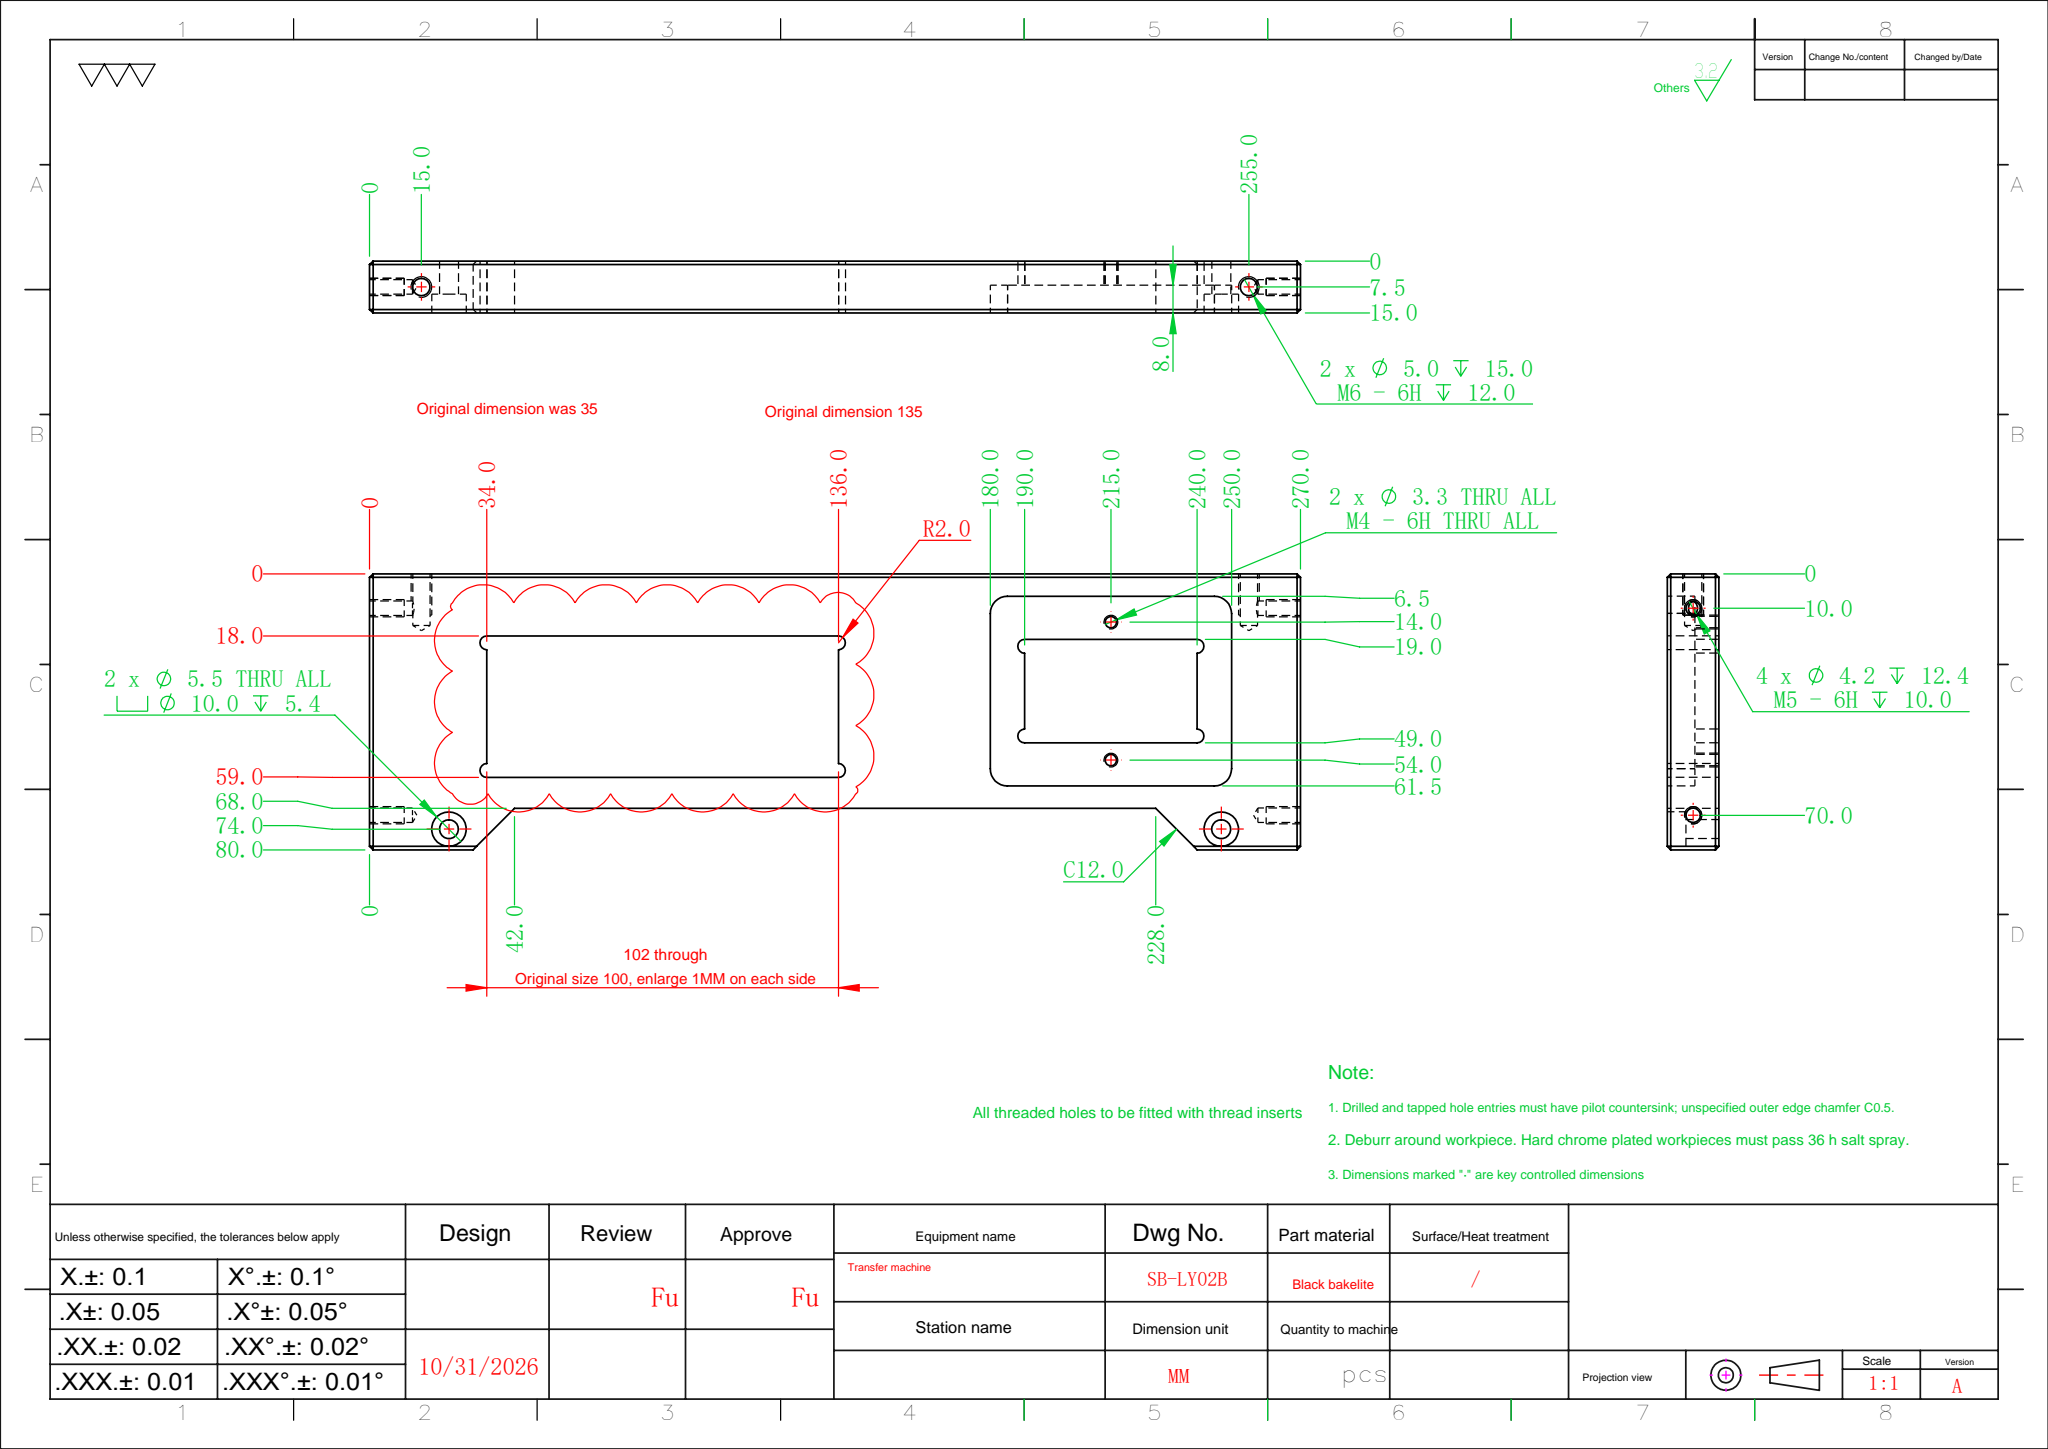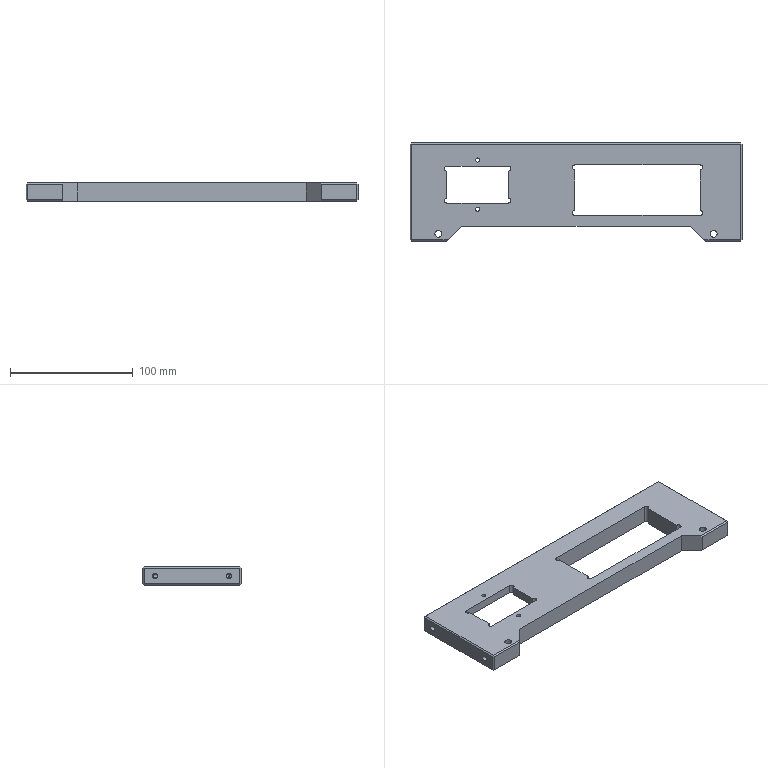Part | SolidWorks | features Cut 4, HoleWzd 4, Chamfer 2, ICE 2, Extrusion 1, Fillet 1, MirrorPattern 1 | 1 solid | 99 faces | box 270 x 80 x 15 mm | volume 180697 mm3 | plane 47 | cylinder 40 | cone 12 | commonest cylinder face diameters 4 x12 4.2 x8 10 x8 3.3 x4 5 x4 5.5 x4